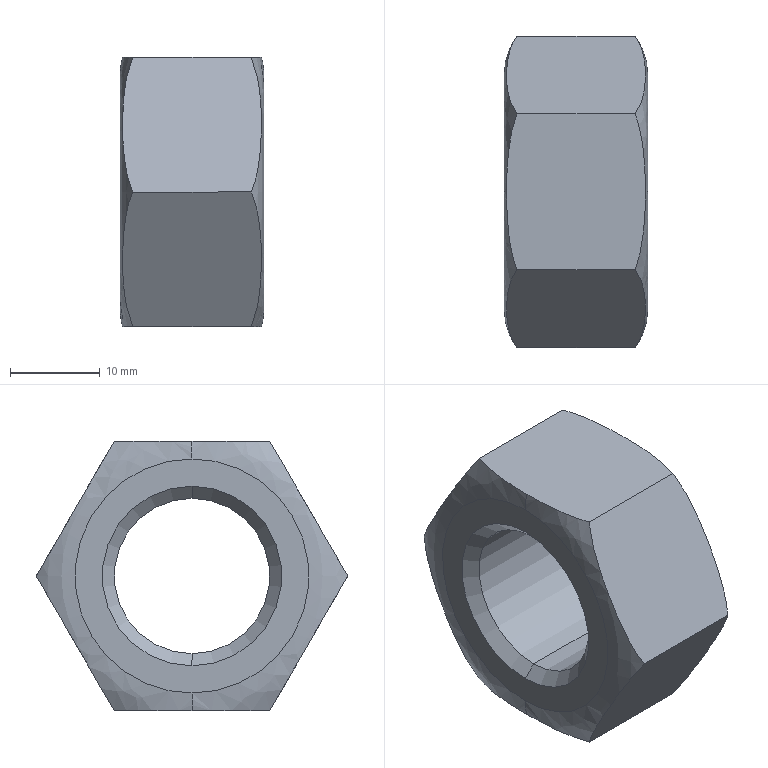Part | SolidWorks | features BaseBody 1 | 1 solid | 18 faces | box 16 x 34.641 x 30 mm | volume 8496 mm3 | plane 8 | spline 4 | cone 4 | cylinder 2 | commonest cylinder face diameters 17.294 x2
STEP:
#1=CARTESIAN_POINT('',(1.401,-8.66,15.));
#2=VERTEX_POINT('',#1);
#3=CARTESIAN_POINT('',(0.2735,0.,15.));
#4=VERTEX_POINT('',#3);
#5=CARTESIAN_POINT('',(1.401,-8.66,15.));
#6=CARTESIAN_POINT('',(1.148,-7.966,15.));
#7=CARTESIAN_POINT('',(0.9589,-7.26,15.));
#8=CARTESIAN_POINT('',(0.6645,-5.832,15.));
#9=CARTESIAN_POINT('',(0.5592,-5.11,15.));
#10=CARTESIAN_POINT('',(0.4034,-3.657,15.));
#11=CARTESIAN_POINT('',(0.3528,-2.924,15.));
#12=CARTESIAN_POINT('',(0.2879,-1.461,15.));
#13=CARTESIAN_POINT('',(0.2735,-0.73,15.));
#14=CARTESIAN_POINT('',(0.2735,0.,15.));
#15=B_SPLINE_CURVE_WITH_KNOTS('',3,(#5,#6,#7,#8,#9,#10,#11,#12,#13,#14),.UNSPECIFIED.,.F.,.F.,(4,2,2,2,4),(0.,0.002186,0.004373,0.006559,0.008745),.UNSPECIFIED.);
#16=EDGE_CURVE('',#2,#4,#15,.T.);
#17=ORIENTED_EDGE('',*,*,#16,.T.);
#18=CARTESIAN_POINT('',(0.,0.,13.021));
#19=VERTEX_POINT('',#18);
#20=CARTESIAN_POINT('',(7.3,0.,13.021));
#21=DIRECTION('',(0.,-1.,0.));
#22=DIRECTION('',(0.,0.,1.));
#23=AXIS2_PLACEMENT_3D('',#20,#21,#22);
#24=CIRCLE('',#23,7.3);
#25=EDGE_CURVE('',#4,#19,#24,.T.);
#26=ORIENTED_EDGE('',*,*,#25,.T.);
#27=CARTESIAN_POINT('',(0.,0.,-13.021));
#28=VERTEX_POINT('',#27);
#29=CARTESIAN_POINT('',(0.,0.,-13.021));
#30=CARTESIAN_POINT('',(0.,-0.3981,-13.021));
#31=CARTESIAN_POINT('',(0.,-0.9928,-12.993));
#32=CARTESIAN_POINT('',(0.,-1.682,-12.914));
#33=CARTESIAN_POINT('',(0.,-2.026,-12.863));
#34=CARTESIAN_POINT('',(0.,-2.198,-12.834));
#35=CARTESIAN_POINT('',(0.,-2.271,-12.821));
#36=CARTESIAN_POINT('',(0.,-2.32,-12.812));
#37=CARTESIAN_POINT('',(0.,-2.343,-12.808));
#38=CARTESIAN_POINT('',(0.,-2.784,-12.726));
#39=CARTESIAN_POINT('',(0.,-3.399,-12.582));
#40=CARTESIAN_POINT('',(0.,-4.101,-12.361));
#41=CARTESIAN_POINT('',(0.,-4.448,-12.238));
#42=CARTESIAN_POINT('',(0.,-4.596,-12.183));
#43=CARTESIAN_POINT('',(0.,-4.694,-12.145));
#44=CARTESIAN_POINT('',(0.,-4.742,-12.127));
#45=CARTESIAN_POINT('',(0.,-5.202,-11.944));
#46=CARTESIAN_POINT('',(0.,-5.8,-11.672));
#47=CARTESIAN_POINT('',(0.,-6.471,-11.302));
#48=CARTESIAN_POINT('',(0.,-6.8,-11.105));
#49=CARTESIAN_POINT('',(0.,-6.94,-11.017));
#50=CARTESIAN_POINT('',(0.,-7.033,-10.958));
#51=CARTESIAN_POINT('',(0.,-7.078,-10.929));
#52=CARTESIAN_POINT('',(0.,-7.877,-10.406));
#53=CARTESIAN_POINT('',(0.,-8.572,-9.842));
#54=CARTESIAN_POINT('',(0.,-9.525,-8.889));
#55=CARTESIAN_POINT('',(0.,-9.974,-8.391));
#56=CARTESIAN_POINT('',(0.,-10.452,-7.771));
#57=CARTESIAN_POINT('',(0.,-10.679,-7.451));
#58=CARTESIAN_POINT('',(0.,-10.774,-7.312));
#59=CARTESIAN_POINT('',(0.,-10.836,-7.219));
#60=CARTESIAN_POINT('',(0.,-10.868,-7.171));
#61=CARTESIAN_POINT('',(0.,-11.139,-6.757));
#62=CARTESIAN_POINT('',(0.,-11.47,-6.189));
#63=CARTESIAN_POINT('',(0.,-11.806,-5.5));
#64=CARTESIAN_POINT('',(0.,-11.96,-5.149));
#65=CARTESIAN_POINT('',(0.,-12.034,-4.971));
#66=CARTESIAN_POINT('',(0.,-12.065,-4.895));
#67=CARTESIAN_POINT('',(0.,-12.086,-4.844));
#68=CARTESIAN_POINT('',(0.,-12.097,-4.817));
#69=CARTESIAN_POINT('',(0.,-12.262,-4.4));
#70=CARTESIAN_POINT('',(0.,-12.465,-3.803));
#71=CARTESIAN_POINT('',(0.,-12.651,-3.091));
#72=CARTESIAN_POINT('',(0.,-12.732,-2.731));
#73=CARTESIAN_POINT('',(0.,-12.768,-2.551));
#74=CARTESIAN_POINT('',(0.,-12.784,-2.473));
#75=CARTESIAN_POINT('',(0.,-12.793,-2.421));
#76=CARTESIAN_POINT('',(0.,-12.799,-2.394));
#77=CARTESIAN_POINT('',(0.,-12.948,-1.587));
#78=CARTESIAN_POINT('',(0.,-13.02,-0.796));
#79=CARTESIAN_POINT('',(0.,-13.021,0.398));
#80=CARTESIAN_POINT('',(0.,-12.993,0.9927));
#81=CARTESIAN_POINT('',(0.,-12.914,1.682));
#82=CARTESIAN_POINT('',(0.,-12.863,2.026));
#83=CARTESIAN_POINT('',(0.,-12.834,2.198));
#84=CARTESIAN_POINT('',(0.,-12.821,2.271));
#85=CARTESIAN_POINT('',(0.,-12.812,2.32));
#86=CARTESIAN_POINT('',(0.,-12.808,2.343));
#87=CARTESIAN_POINT('',(0.,-12.726,2.784));
#88=CARTESIAN_POINT('',(0.,-12.582,3.399));
#89=CARTESIAN_POINT('',(0.,-12.361,4.101));
#90=CARTESIAN_POINT('',(0.,-12.238,4.448));
#91=CARTESIAN_POINT('',(0.,-12.183,4.596));
#92=CARTESIAN_POINT('',(0.,-12.145,4.694));
#93=CARTESIAN_POINT('',(0.,-12.127,4.742));
#94=CARTESIAN_POINT('',(0.,-11.944,5.202));
#95=CARTESIAN_POINT('',(0.,-11.672,5.8));
#96=CARTESIAN_POINT('',(0.,-11.302,6.471));
#97=CARTESIAN_POINT('',(0.,-11.105,6.8));
#98=CARTESIAN_POINT('',(0.,-11.017,6.94));
#99=CARTESIAN_POINT('',(0.,-10.958,7.033));
#100=CARTESIAN_POINT('',(0.,-10.929,7.078));
#101=CARTESIAN_POINT('',(0.,-10.406,7.877));
#102=CARTESIAN_POINT('',(0.,-9.842,8.572));
#103=CARTESIAN_POINT('',(0.,-8.889,9.525));
#104=CARTESIAN_POINT('',(0.,-8.391,9.974));
#105=CARTESIAN_POINT('',(0.,-7.771,10.452));
#106=CARTESIAN_POINT('',(0.,-7.451,10.679));
#107=CARTESIAN_POINT('',(0.,-7.312,10.774));
#108=CARTESIAN_POINT('',(0.,-7.219,10.836));
#109=CARTESIAN_POINT('',(0.,-7.171,10.868));
#110=CARTESIAN_POINT('',(0.,-6.757,11.139));
#111=CARTESIAN_POINT('',(0.,-6.189,11.47));
#112=CARTESIAN_POINT('',(0.,-5.5,11.806));
#113=CARTESIAN_POINT('',(0.,-5.149,11.96));
#114=CARTESIAN_POINT('',(0.,-4.971,12.034));
#115=CARTESIAN_POINT('',(0.,-4.895,12.065));
#116=CARTESIAN_POINT('',(0.,-4.844,12.086));
#117=CARTESIAN_POINT('',(0.,-4.817,12.097));
#118=CARTESIAN_POINT('',(0.,-4.4,12.262));
#119=CARTESIAN_POINT('',(0.,-3.803,12.465));
#120=CARTESIAN_POINT('',(0.,-3.091,12.651));
#121=CARTESIAN_POINT('',(0.,-2.731,12.732));
#122=CARTESIAN_POINT('',(0.,-2.551,12.768));
#123=CARTESIAN_POINT('',(0.,-2.473,12.784));
#124=CARTESIAN_POINT('',(0.,-2.421,12.793));
#125=CARTESIAN_POINT('',(0.,-2.394,12.799));
#126=CARTESIAN_POINT('',(0.,-1.587,12.948));
#127=CARTESIAN_POINT('',(0.,-0.796,13.02));
#128=CARTESIAN_POINT('',(0.,0.,13.021));
#129=B_SPLINE_CURVE_WITH_KNOTS('',3,(#29,#30,#31,#32,#33,#34,#35,#36,#37,#38,#39,#40,#41,#42,#43,#44,#45,#46,#47,#48,#49,#50,#51,#52,#53,#54,#55,#56,#57,#58,#59,#60,#61,#62,#63,#64,#65,#66,#67,#68,#69,#70,#71,#72,#73,#74,#75,#76,#77,#78,#79,#80,#81,#82,#83,#84,#85,#86,#87,#88,#89,#90,#91,#92,#93,#94,#95,#96,#97,#98,#99,#100,#101,#102,#103,#104,#105,#106,#107,#108,#109,#110,#111,#112,#113,#114,#115,#116,#117,#118,#119,#120,#121,#122,#123,#124,#125,#126,#127,#128),.UNSPECIFIED.,.F.,.F.,(4,1,1,1,1,2,2,1,1,1,2,2,1,1,1,2,2,2,1,1,1,2,2,1,1,1,1,2,2,1,1,1,1,2,2,2,1,1,1,1,2,2,1,1,1,2,2,1,1,1,2,2,2,1,1,1,2,2,1,1,1,1,2,2,1,1,1,1,2,2,4),(0.,0.01563,0.02344,0.02734,0.0293,0.03027,0.03125,0.04688,0.05469,0.05859,0.06055,0.0625,0.07813,0.08594,0.08984,0.0918,0.09375,0.125,0.1406,0.1484,0.1523,0.1543,0.1563,0.1719,0.1797,0.1836,0.1855,0.1865,0.1875,0.2031,0.2109,0.2148,0.2168,0.2178,0.2188,0.25,0.2656,0.2734,0.2773,0.2793,0.2803,0.2813,0.2969,0.3047,0.3086,0.3105,0.3125,0.3281,0.3359,0.3398,0.3418,0.3438,0.375,0.3906,0.3984,0.4023,0.4043,0.4063,0.4219,0.4297,0.4336,0.4355,0.4365,0.4375,0.4531,0.4609,0.4648,0.4668,0.4678,0.4688,0.5),.UNSPECIFIED.);
#130=EDGE_CURVE('',#28,#19,#129,.T.);
#131=ORIENTED_EDGE('',*,*,#130,.F.);
#132=CARTESIAN_POINT('',(0.2735,0.,-15.));
#133=VERTEX_POINT('',#132);
#134=CARTESIAN_POINT('',(7.3,0.,-13.021));
#135=DIRECTION('',(0.,1.,0.));
#136=DIRECTION('',(0.,0.,-1.));
#137=AXIS2_PLACEMENT_3D('',#134,#135,#136);
#138=CIRCLE('',#137,7.3);
#139=EDGE_CURVE('',#133,#28,#138,.T.);
#140=ORIENTED_EDGE('',*,*,#139,.F.);
#141=CARTESIAN_POINT('',(1.401,-8.66,-15.));
#142=VERTEX_POINT('',#141);
#143=CARTESIAN_POINT('',(0.2735,0.,-15.));
#144=CARTESIAN_POINT('',(0.2735,-0.7289,-15.));
#145=CARTESIAN_POINT('',(0.2879,-1.457,-15.));
#146=CARTESIAN_POINT('',(0.3521,-2.912,-15.));
#147=CARTESIAN_POINT('',(0.4019,-3.638,-15.));
#148=CARTESIAN_POINT('',(0.5565,-5.089,-15.));
#149=CARTESIAN_POINT('',(0.6611,-5.813,-15.));
#150=CARTESIAN_POINT('',(0.9579,-7.257,-15.));
#151=CARTESIAN_POINT('',(1.148,-7.967,-15.));
#152=CARTESIAN_POINT('',(1.401,-8.66,-15.));
#153=B_SPLINE_CURVE_WITH_KNOTS('',3,(#143,#144,#145,#146,#147,#148,#149,#150,#151,#152),.UNSPECIFIED.,.F.,.F.,(4,2,2,2,4),(0.008745,0.01093,0.01311,0.01529,0.01748),.UNSPECIFIED.);
#154=EDGE_CURVE('',#133,#142,#153,.T.);
#155=ORIENTED_EDGE('',*,*,#154,.T.);
#156=CARTESIAN_POINT('',(1.401,-17.321,0.));
#157=VERTEX_POINT('',#156);
#158=CARTESIAN_POINT('',(1.401,-8.66,-15.));
#159=CARTESIAN_POINT('',(1.148,-9.007,-14.399));
#160=CARTESIAN_POINT('',(0.9592,-9.36,-13.788));
#161=CARTESIAN_POINT('',(0.6649,-10.073,-12.552));
#162=CARTESIAN_POINT('',(0.5596,-10.434,-11.928));
#163=CARTESIAN_POINT('',(0.4037,-11.16,-10.67));
#164=CARTESIAN_POINT('',(0.3531,-11.526,-10.036));
#165=CARTESIAN_POINT('',(0.2881,-12.257,-8.77));
#166=CARTESIAN_POINT('',(0.2736,-12.622,-8.138));
#167=CARTESIAN_POINT('',(0.2734,-13.352,-6.874));
#168=CARTESIAN_POINT('',(0.2878,-13.716,-6.243));
#169=CARTESIAN_POINT('',(0.3518,-14.444,-4.982));
#170=CARTESIAN_POINT('',(0.4016,-14.808,-4.353));
#171=CARTESIAN_POINT('',(0.5561,-15.533,-3.095));
#172=CARTESIAN_POINT('',(0.6607,-15.896,-2.468));
#173=CARTESIAN_POINT('',(0.9576,-16.618,-1.216));
#174=CARTESIAN_POINT('',(1.148,-16.974,-0.6006));
#175=CARTESIAN_POINT('',(1.401,-17.321,0.));
#176=B_SPLINE_CURVE_WITH_KNOTS('',3,(#158,#159,#160,#161,#162,#163,#164,#165,#166,#167,#168,#169,#170,#171,#172,#173,#174,#175),.UNSPECIFIED.,.F.,.F.,(4,2,2,2,2,2,2,2,4),(0.,0.002185,0.004369,0.006554,0.008739,0.01092,0.01311,0.01529,0.01748),.UNSPECIFIED.);
#177=EDGE_CURVE('',#142,#157,#176,.T.);
#178=ORIENTED_EDGE('',*,*,#177,.T.);
#179=CARTESIAN_POINT('',(1.401,-17.321,0.));
#180=CARTESIAN_POINT('',(1.148,-16.974,0.6009));
#181=CARTESIAN_POINT('',(0.9592,-16.621,1.212));
#182=CARTESIAN_POINT('',(0.6649,-15.907,2.448));
#183=CARTESIAN_POINT('',(0.5596,-15.547,3.072));
#184=CARTESIAN_POINT('',(0.4037,-14.821,4.33));
#185=CARTESIAN_POINT('',(0.3531,-14.454,4.964));
#186=CARTESIAN_POINT('',(0.2881,-13.723,6.23));
#187=CARTESIAN_POINT('',(0.2736,-13.358,6.862));
#188=CARTESIAN_POINT('',(0.2734,-12.629,8.126));
#189=CARTESIAN_POINT('',(0.2878,-12.265,8.757));
#190=CARTESIAN_POINT('',(0.3518,-11.537,10.018));
#191=CARTESIAN_POINT('',(0.4016,-11.173,10.647));
#192=CARTESIAN_POINT('',(0.5561,-10.447,11.905));
#193=CARTESIAN_POINT('',(0.6607,-10.085,12.532));
#194=CARTESIAN_POINT('',(0.9576,-9.363,13.784));
#195=CARTESIAN_POINT('',(1.148,-9.007,14.399));
#196=CARTESIAN_POINT('',(1.401,-8.66,15.));
#197=B_SPLINE_CURVE_WITH_KNOTS('',3,(#179,#180,#181,#182,#183,#184,#185,#186,#187,#188,#189,#190,#191,#192,#193,#194,#195,#196),.UNSPECIFIED.,.F.,.F.,(4,2,2,2,2,2,2,2,4),(0.,0.002185,0.004369,0.006554,0.008739,0.01092,0.01311,0.01529,0.01748),.UNSPECIFIED.);
#198=EDGE_CURVE('',#157,#2,#197,.T.);
#199=ORIENTED_EDGE('',*,*,#198,.T.);
#200=EDGE_LOOP('',(#17,#26,#131,#140,#155,#178,#199));
#201=FACE_OUTER_BOUND('',#200,.T.);
#202=CARTESIAN_POINT('',(1.417,0.,17.343));
#203=CARTESIAN_POINT('',(1.417,-34.686,17.343));
#204=CARTESIAN_POINT('',(1.417,-34.686,-17.343));
#205=CARTESIAN_POINT('',(1.417,0.,-17.343));
#206=CARTESIAN_POINT('',(0.4886,0.,16.079));
#207=CARTESIAN_POINT('',(0.4886,-32.158,16.079));
#208=CARTESIAN_POINT('',(0.4886,-32.158,-16.079));
#209=CARTESIAN_POINT('',(0.4886,0.,-16.079));
#210=CARTESIAN_POINT('',(0.,0.,14.589));
#211=CARTESIAN_POINT('',(0.,-29.178,14.589));
#212=CARTESIAN_POINT('',(0.,-29.178,-14.589));
#213=CARTESIAN_POINT('',(0.,0.,-14.589));
#214=CARTESIAN_POINT('',(0.,0.,13.021));
#215=CARTESIAN_POINT('',(0.,-26.041,13.021));
#216=CARTESIAN_POINT('',(0.,-26.041,-13.021));
#217=CARTESIAN_POINT('',(0.,0.,-13.021));
#218=(BOUNDED_SURFACE()B_SPLINE_SURFACE(3,3,((#202,#203,#204,#205),(#206,#207,#208,#209),(#210,#211,#212,#213),(#214,#215,#216,#217)),.UNSPECIFIED.,.F.,.F.,.F.)B_SPLINE_SURFACE_WITH_KNOTS((4,4),(4,4),(0.,1.),(0.,1.),.UNSPECIFIED.)GEOMETRIC_REPRESENTATION_ITEM()RATIONAL_B_SPLINE_SURFACE(((1.,0.3333,0.3333,1.),(0.9668,0.3223,0.3223,0.9668),(0.9668,0.3223,0.3223,0.9668),(1.,0.3333,0.3333,1.)))REPRESENTATION_ITEM('')SURFACE());
#219=ADVANCED_FACE('',(#201),#218,.T.);
#220=CARTESIAN_POINT('',(16.,0.,13.021));
#221=VERTEX_POINT('',#220);
#222=CARTESIAN_POINT('',(16.,0.,-13.021));
#223=VERTEX_POINT('',#222);
#224=CARTESIAN_POINT('',(16.,0.,13.021));
#225=CARTESIAN_POINT('',(16.,-0.398,13.021));
#226=CARTESIAN_POINT('',(16.,-0.9927,12.993));
#227=CARTESIAN_POINT('',(16.,-1.682,12.914));
#228=CARTESIAN_POINT('',(16.,-2.026,12.863));
#229=CARTESIAN_POINT('',(16.,-2.198,12.834));
#230=CARTESIAN_POINT('',(16.,-2.271,12.821));
#231=CARTESIAN_POINT('',(16.,-2.32,12.812));
#232=CARTESIAN_POINT('',(16.,-2.343,12.808));
#233=CARTESIAN_POINT('',(16.,-2.784,12.726));
#234=CARTESIAN_POINT('',(16.,-3.399,12.582));
#235=CARTESIAN_POINT('',(16.,-4.101,12.361));
#236=CARTESIAN_POINT('',(16.,-4.448,12.238));
#237=CARTESIAN_POINT('',(16.,-4.596,12.183));
#238=CARTESIAN_POINT('',(16.,-4.694,12.145));
#239=CARTESIAN_POINT('',(16.,-4.742,12.127));
#240=CARTESIAN_POINT('',(16.,-5.202,11.944));
#241=CARTESIAN_POINT('',(16.,-5.8,11.672));
#242=CARTESIAN_POINT('',(16.,-6.471,11.302));
#243=CARTESIAN_POINT('',(16.,-6.8,11.105));
#244=CARTESIAN_POINT('',(16.,-6.94,11.017));
#245=CARTESIAN_POINT('',(16.,-7.033,10.958));
#246=CARTESIAN_POINT('',(16.,-7.078,10.929));
#247=CARTESIAN_POINT('',(16.,-7.877,10.406));
#248=CARTESIAN_POINT('',(16.,-8.572,9.842));
#249=CARTESIAN_POINT('',(16.,-9.525,8.889));
#250=CARTESIAN_POINT('',(16.,-9.974,8.391));
#251=CARTESIAN_POINT('',(16.,-10.452,7.771));
#252=CARTESIAN_POINT('',(16.,-10.679,7.451));
#253=CARTESIAN_POINT('',(16.,-10.774,7.312));
#254=CARTESIAN_POINT('',(16.,-10.836,7.219));
#255=CARTESIAN_POINT('',(16.,-10.868,7.171));
#256=CARTESIAN_POINT('',(16.,-11.139,6.757));
#257=CARTESIAN_POINT('',(16.,-11.47,6.189));
#258=CARTESIAN_POINT('',(16.,-11.806,5.5));
#259=CARTESIAN_POINT('',(16.,-11.96,5.149));
#260=CARTESIAN_POINT('',(16.,-12.034,4.971));
#261=CARTESIAN_POINT('',(16.,-12.065,4.895));
#262=CARTESIAN_POINT('',(16.,-12.086,4.844));
#263=CARTESIAN_POINT('',(16.,-12.097,4.817));
#264=CARTESIAN_POINT('',(16.,-12.262,4.4));
#265=CARTESIAN_POINT('',(16.,-12.465,3.803));
#266=CARTESIAN_POINT('',(16.,-12.651,3.091));
#267=CARTESIAN_POINT('',(16.,-12.732,2.731));
#268=CARTESIAN_POINT('',(16.,-12.768,2.551));
#269=CARTESIAN_POINT('',(16.,-12.784,2.473));
#270=CARTESIAN_POINT('',(16.,-12.793,2.421));
#271=CARTESIAN_POINT('',(16.,-12.799,2.394));
#272=CARTESIAN_POINT('',(16.,-12.948,1.587));
#273=CARTESIAN_POINT('',(16.,-13.02,0.796));
#274=CARTESIAN_POINT('',(16.,-13.021,-0.398));
#275=CARTESIAN_POINT('',(16.,-12.993,-0.9927));
#276=CARTESIAN_POINT('',(16.,-12.914,-1.682));
#277=CARTESIAN_POINT('',(16.,-12.863,-2.026));
#278=CARTESIAN_POINT('',(16.,-12.834,-2.198));
#279=CARTESIAN_POINT('',(16.,-12.821,-2.271));
#280=CARTESIAN_POINT('',(16.,-12.812,-2.32));
#281=CARTESIAN_POINT('',(16.,-12.808,-2.343));
#282=CARTESIAN_POINT('',(16.,-12.726,-2.784));
#283=CARTESIAN_POINT('',(16.,-12.582,-3.399));
#284=CARTESIAN_POINT('',(16.,-12.361,-4.101));
#285=CARTESIAN_POINT('',(16.,-12.238,-4.448));
#286=CARTESIAN_POINT('',(16.,-12.183,-4.596));
#287=CARTESIAN_POINT('',(16.,-12.145,-4.694));
#288=CARTESIAN_POINT('',(16.,-12.127,-4.742));
#289=CARTESIAN_POINT('',(16.,-11.944,-5.202));
#290=CARTESIAN_POINT('',(16.,-11.672,-5.8));
#291=CARTESIAN_POINT('',(16.,-11.302,-6.471));
#292=CARTESIAN_POINT('',(16.,-11.105,-6.8));
#293=CARTESIAN_POINT('',(16.,-11.017,-6.94));
#294=CARTESIAN_POINT('',(16.,-10.958,-7.033));
#295=CARTESIAN_POINT('',(16.,-10.929,-7.078));
#296=CARTESIAN_POINT('',(16.,-10.406,-7.877));
#297=CARTESIAN_POINT('',(16.,-9.842,-8.572));
#298=CARTESIAN_POINT('',(16.,-8.889,-9.525));
#299=CARTESIAN_POINT('',(16.,-8.391,-9.974));
#300=CARTESIAN_POINT('',(16.,-7.771,-10.452));
#301=CARTESIAN_POINT('',(16.,-7.451,-10.679));
#302=CARTESIAN_POINT('',(16.,-7.312,-10.774));
#303=CARTESIAN_POINT('',(16.,-7.219,-10.836));
#304=CARTESIAN_POINT('',(16.,-7.171,-10.868));
#305=CARTESIAN_POINT('',(16.,-6.757,-11.139));
#306=CARTESIAN_POINT('',(16.,-6.189,-11.47));
#307=CARTESIAN_POINT('',(16.,-5.5,-11.806));
#308=CARTESIAN_POINT('',(16.,-5.149,-11.96));
#309=CARTESIAN_POINT('',(16.,-4.971,-12.034));
#310=CARTESIAN_POINT('',(16.,-4.895,-12.065));
#311=CARTESIAN_POINT('',(16.,-4.844,-12.086));
#312=CARTESIAN_POINT('',(16.,-4.817,-12.097));
#313=CARTESIAN_POINT('',(16.,-4.4,-12.262));
#314=CARTESIAN_POINT('',(16.,-3.803,-12.465));
#315=CARTESIAN_POINT('',(16.,-3.091,-12.651));
#316=CARTESIAN_POINT('',(16.,-2.731,-12.732));
#317=CARTESIAN_POINT('',(16.,-2.551,-12.768));
#318=CARTESIAN_POINT('',(16.,-2.473,-12.784));
#319=CARTESIAN_POINT('',(16.,-2.421,-12.793));
#320=CARTESIAN_POINT('',(16.,-2.394,-12.799));
#321=CARTESIAN_POINT('',(16.,-1.586,-12.948));
#322=CARTESIAN_POINT('',(16.,-0.7966,-13.021));
#323=CARTESIAN_POINT('',(16.,0.,-13.021));
#324=B_SPLINE_CURVE_WITH_KNOTS('',3,(#224,#225,#226,#227,#228,#229,#230,#231,#232,#233,#234,#235,#236,#237,#238,#239,#240,#241,#242,#243,#244,#245,#246,#247,#248,#249,#250,#251,#252,#253,#254,#255,#256,#257,#258,#259,#260,#261,#262,#263,#264,#265,#266,#267,#268,#269,#270,#271,#272,#273,#274,#275,#276,#277,#278,#279,#280,#281,#282,#283,#284,#285,#286,#287,#288,#289,#290,#291,#292,#293,#294,#295,#296,#297,#298,#299,#300,#301,#302,#303,#304,#305,#306,#307,#308,#309,#310,#311,#312,#313,#314,#315,#316,#317,#318,#319,#320,#321,#322,#323),.UNSPECIFIED.,.F.,.F.,(4,1,1,1,1,2,2,1,1,1,2,2,1,1,1,2,2,2,1,1,1,2,2,1,1,1,1,2,2,1,1,1,1,2,2,2,1,1,1,1,2,2,1,1,1,2,2,1,1,1,2,2,2,1,1,1,2,2,1,1,1,1,2,2,1,1,1,1,2,2,4),(0.5,0.5156,0.5234,0.5273,0.5293,0.5303,0.5312,0.5469,0.5547,0.5586,0.5605,0.5625,0.5781,0.5859,0.5898,0.5918,0.5937,0.625,0.6406,0.6484,0.6523,0.6543,0.6562,0.6719,0.6797,0.6836,0.6855,0.6865,0.6875,0.7031,0.7109,0.7148,0.7168,0.7178,0.7187,0.75,0.7656,0.7734,0.7773,0.7793,0.7803,0.7812,0.7969,0.8047,0.8086,0.8105,0.8125,0.8281,0.8359,0.8398,0.8418,0.8437,0.875,0.8906,0.8984,0.9023,0.9043,0.9062,0.9219,0.9297,0.9336,0.9355,0.9365,0.9375,0.9531,0.9609,0.9648,0.9668,0.9678,0.9687,1.),.UNSPECIFIED.);
#325=EDGE_CURVE('',#221,#223,#324,.T.);
#326=ORIENTED_EDGE('',*,*,#325,.F.);
#327=CARTESIAN_POINT('',(15.726,0.,15.));
#328=VERTEX_POINT('',#327);
#329=CARTESIAN_POINT('',(8.7,0.,13.021));
#330=DIRECTION('',(0.,-1.,0.));
#331=DIRECTION('',(0.,0.,1.));
#332=AXIS2_PLACEMENT_3D('',#329,#330,#331);
#333=CIRCLE('',#332,7.3);
#334=EDGE_CURVE('',#221,#328,#333,.T.);
#335=ORIENTED_EDGE('',*,*,#334,.T.);
#336=CARTESIAN_POINT('',(14.599,-8.66,15.));
#337=VERTEX_POINT('',#336);
#338=CARTESIAN_POINT('',(15.726,0.,15.));
#339=CARTESIAN_POINT('',(15.726,-0.7289,15.));
#340=CARTESIAN_POINT('',(15.712,-1.457,15.));
#341=CARTESIAN_POINT('',(15.648,-2.912,15.));
#342=CARTESIAN_POINT('',(15.598,-3.638,15.));
#343=CARTESIAN_POINT('',(15.444,-5.089,15.));
#344=CARTESIAN_POINT('',(15.339,-5.813,15.));
#345=CARTESIAN_POINT('',(15.042,-7.257,15.));
#346=CARTESIAN_POINT('',(14.852,-7.967,15.));
#347=CARTESIAN_POINT('',(14.599,-8.66,15.));
#348=B_SPLINE_CURVE_WITH_KNOTS('',3,(#338,#339,#340,#341,#342,#343,#344,#345,#346,#347),.UNSPECIFIED.,.F.,.F.,(4,2,2,2,4),(0.008745,0.01093,0.01311,0.01529,0.01748),.UNSPECIFIED.);
#349=EDGE_CURVE('',#328,#337,#348,.T.);
#350=ORIENTED_EDGE('',*,*,#349,.T.);
#351=CARTESIAN_POINT('',(14.599,-17.321,0.));
#352=VERTEX_POINT('',#351);
#353=CARTESIAN_POINT('',(14.599,-8.66,15.));
#354=CARTESIAN_POINT('',(14.852,-9.007,14.399));
#355=CARTESIAN_POINT('',(15.041,-9.36,13.788));
#356=CARTESIAN_POINT('',(15.335,-10.073,12.552));
#357=CARTESIAN_POINT('',(15.44,-10.434,11.928));
#358=CARTESIAN_POINT('',(15.596,-11.16,10.67));
#359=CARTESIAN_POINT('',(15.647,-11.526,10.036));
#360=CARTESIAN_POINT('',(15.712,-12.257,8.77));
#361=CARTESIAN_POINT('',(15.726,-12.622,8.138));
#362=CARTESIAN_POINT('',(15.727,-13.352,6.874));
#363=CARTESIAN_POINT('',(15.712,-13.716,6.243));
#364=CARTESIAN_POINT('',(15.648,-14.444,4.982));
#365=CARTESIAN_POINT('',(15.598,-14.808,4.353));
#366=CARTESIAN_POINT('',(15.444,-15.533,3.095));
#367=CARTESIAN_POINT('',(15.339,-15.896,2.468));
#368=CARTESIAN_POINT('',(15.042,-16.618,1.216));
#369=CARTESIAN_POINT('',(14.852,-16.974,0.6006));
#370=CARTESIAN_POINT('',(14.599,-17.321,0.));
#371=B_SPLINE_CURVE_WITH_KNOTS('',3,(#353,#354,#355,#356,#357,#358,#359,#360,#361,#362,#363,#364,#365,#366,#367,#368,#369,#370),.UNSPECIFIED.,.F.,.F.,(4,2,2,2,2,2,2,2,4),(0.,0.002185,0.004369,0.006554,0.008739,0.01092,0.01311,0.01529,0.01748),.UNSPECIFIED.);
#372=EDGE_CURVE('',#337,#352,#371,.T.);
#373=ORIENTED_EDGE('',*,*,#372,.T.);
#374=CARTESIAN_POINT('',(14.599,-8.66,-15.));
#375=VERTEX_POINT('',#374);
#376=CARTESIAN_POINT('',(14.599,-17.321,0.));
#377=CARTESIAN_POINT('',(14.852,-16.974,-0.6009));
#378=CARTESIAN_POINT('',(15.041,-16.621,-1.212));
#379=CARTESIAN_POINT('',(15.335,-15.907,-2.448));
#380=CARTESIAN_POINT('',(15.44,-15.547,-3.072));
#381=CARTESIAN_POINT('',(15.596,-14.821,-4.33));
#382=CARTESIAN_POINT('',(15.647,-14.454,-4.964));
#383=CARTESIAN_POINT('',(15.712,-13.723,-6.23));
#384=CARTESIAN_POINT('',(15.726,-13.358,-6.862));
#385=CARTESIAN_POINT('',(15.727,-12.629,-8.126));
#386=CARTESIAN_POINT('',(15.712,-12.265,-8.757));
#387=CARTESIAN_POINT('',(15.648,-11.537,-10.018));
#388=CARTESIAN_POINT('',(15.598,-11.173,-10.647));
#389=CARTESIAN_POINT('',(15.444,-10.447,-11.905));
#390=CARTESIAN_POINT('',(15.339,-10.085,-12.532));
#391=CARTESIAN_POINT('',(15.042,-9.363,-13.784));
#392=CARTESIAN_POINT('',(14.852,-9.007,-14.399));
#393=CARTESIAN_POINT('',(14.599,-8.66,-15.));
#394=B_SPLINE_CURVE_WITH_KNOTS('',3,(#376,#377,#378,#379,#380,#381,#382,#383,#384,#385,#386,#387,#388,#389,#390,#391,#392,#393),.UNSPECIFIED.,.F.,.F.,(4,2,2,2,2,2,2,2,4),(0.,0.002185,0.004369,0.006554,0.008739,0.01092,0.01311,0.01529,0.01748),.UNSPECIFIED.);
#395=EDGE_CURVE('',#352,#375,#394,.T.);
#396=ORIENTED_EDGE('',*,*,#395,.T.);
#397=CARTESIAN_POINT('',(15.726,0.,-15.));
#398=VERTEX_POINT('',#397);
#399=CARTESIAN_POINT('',(14.599,-8.66,-15.));
#400=CARTESIAN_POINT('',(14.852,-7.966,-15.));
#401=CARTESIAN_POINT('',(15.041,-7.26,-15.));
#402=CARTESIAN_POINT('',(15.336,-5.832,-15.));
#403=CARTESIAN_POINT('',(15.441,-5.11,-15.));
#404=CARTESIAN_POINT('',(15.597,-3.657,-15.));
#405=CARTESIAN_POINT('',(15.647,-2.924,-15.));
#406=CARTESIAN_POINT('',(15.712,-1.461,-15.));
#407=CARTESIAN_POINT('',(15.726,-0.73,-15.));
#408=CARTESIAN_POINT('',(15.726,0.,-15.));
#409=B_SPLINE_CURVE_WITH_KNOTS('',3,(#399,#400,#401,#402,#403,#404,#405,#406,#407,#408),.UNSPECIFIED.,.F.,.F.,(4,2,2,2,4),(0.,0.002186,0.004373,0.006559,0.008745),.UNSPECIFIED.);
#410=EDGE_CURVE('',#375,#398,#409,.T.);
#411=ORIENTED_EDGE('',*,*,#410,.T.);
#412=CARTESIAN_POINT('',(8.7,0.,-13.021));
#413=DIRECTION('',(0.,1.,0.));
#414=DIRECTION('',(0.,0.,-1.));
#415=AXIS2_PLACEMENT_3D('',#412,#413,#414);
#416=CIRCLE('',#415,7.3);
#417=EDGE_CURVE('',#223,#398,#416,.T.);
#418=ORIENTED_EDGE('',*,*,#417,.F.);
#419=EDGE_LOOP('',(#326,#335,#350,#373,#396,#411,#418));
#420=FACE_OUTER_BOUND('',#419,.T.);
#421=CARTESIAN_POINT('',(16.,0.,13.021));
#422=CARTESIAN_POINT('',(16.,-26.041,13.021));
#423=CARTESIAN_POINT('',(16.,-26.041,-13.021));
#424=CARTESIAN_POINT('',(16.,0.,-13.021));
#425=CARTESIAN_POINT('',(16.,0.,14.589));
#426=CARTESIAN_POINT('',(16.,-29.178,14.589));
#427=CARTESIAN_POINT('',(16.,-29.178,-14.589));
#428=CARTESIAN_POINT('',(16.,0.,-14.589));
#429=CARTESIAN_POINT('',(15.511,0.,16.079));
#430=CARTESIAN_POINT('',(15.511,-32.158,16.079));
#431=CARTESIAN_POINT('',(15.511,-32.158,-16.079));
#432=CARTESIAN_POINT('',(15.511,0.,-16.079));
#433=CARTESIAN_POINT('',(14.583,0.,17.343));
#434=CARTESIAN_POINT('',(14.583,-34.686,17.343));
#435=CARTESIAN_POINT('',(14.583,-34.686,-17.343));
#436=CARTESIAN_POINT('',(14.583,0.,-17.343));
#437=(BOUNDED_SURFACE()B_SPLINE_SURFACE(3,3,((#421,#422,#423,#424),(#425,#426,#427,#428),(#429,#430,#431,#432),(#433,#434,#435,#436)),.UNSPECIFIED.,.F.,.F.,.F.)B_SPLINE_SURFACE_WITH_KNOTS((4,4),(4,4),(0.,1.),(0.,1.),.UNSPECIFIED.)GEOMETRIC_REPRESENTATION_ITEM()RATIONAL_B_SPLINE_SURFACE(((1.,0.3333,0.3333,1.),(0.9668,0.3223,0.3223,0.9668),(0.9668,0.3223,0.3223,0.9668),(1.,0.3333,0.3333,1.)))REPRESENTATION_ITEM('')SURFACE());
#438=ADVANCED_FACE('',(#420),#437,.T.);
#439=CARTESIAN_POINT('',(1.353,0.,8.647));
#440=VERTEX_POINT('',#439);
#441=CARTESIAN_POINT('',(1.353,0.,-8.647));
#442=VERTEX_POINT('',#441);
#443=CARTESIAN_POINT('',(1.353,0.,0.));
#444=DIRECTION('',(1.,0.,0.));
#445=DIRECTION('',(0.,0.,-1.));
#446=AXIS2_PLACEMENT_3D('',#443,#444,#445);
#447=CIRCLE('',#446,8.647);
#448=EDGE_CURVE('',#440,#442,#447,.T.);
#449=ORIENTED_EDGE('',*,*,#448,.F.);
#450=CARTESIAN_POINT('',(14.647,0.,8.647));
#451=VERTEX_POINT('',#450);
#452=CARTESIAN_POINT('',(34225.,0.,8.647));
#453=DIRECTION('',(1.,0.,0.));
#454=VECTOR('',#453,1000.);
#455=LINE('',#452,#454);
#456=EDGE_CURVE('',#440,#451,#455,.T.);
#457=ORIENTED_EDGE('',*,*,#456,.T.);
#458=CARTESIAN_POINT('',(14.647,0.,-8.647));
#459=VERTEX_POINT('',#458);
#460=CARTESIAN_POINT('',(14.647,0.,0.));
#461=DIRECTION('',(-1.,0.,0.));
#462=DIRECTION('',(0.,0.,-1.));
#463=AXIS2_PLACEMENT_3D('',#460,#461,#462);
#464=CIRCLE('',#463,8.647);
#465=EDGE_CURVE('',#459,#451,#464,.T.);
#466=ORIENTED_EDGE('',*,*,#465,.F.);
#467=CARTESIAN_POINT('',(34225.,0.,-8.647));
#468=DIRECTION('',(1.,0.,0.));
#469=VECTOR('',#468,1000.);
#470=LINE('',#467,#469);
#471=EDGE_CURVE('',#442,#459,#470,.T.);
#472=ORIENTED_EDGE('',*,*,#471,.F.);
#473=EDGE_LOOP('',(#449,#457,#466,#472));
#474=FACE_OUTER_BOUND('',#473,.T.);
#475=CARTESIAN_POINT('',(34225.,0.,0.));
#476=DIRECTION('',(1.,0.,0.));
#477=DIRECTION('',(0.,0.,-1.));
#478=AXIS2_PLACEMENT_3D('',#475,#476,#477);
#479=CYLINDRICAL_SURFACE('',#478,8.647);
#480=ADVANCED_FACE('',(#474),#479,.F.);
#481=ORIENTED_EDGE('',*,*,#448,.T.);
#482=CARTESIAN_POINT('',(0.,0.,-10.));
#483=VERTEX_POINT('',#482);
#484=CARTESIAN_POINT('',(0.,0.,-10.));
#485=DIRECTION('',(-0.7071,0.,-0.7071));
#486=VECTOR('',#485,1000.);
#487=LINE('',#484,#486);
#488=EDGE_CURVE('',#442,#483,#487,.T.);
#489=ORIENTED_EDGE('',*,*,#488,.T.);
#490=CARTESIAN_POINT('',(0.,0.,10.));
#491=VERTEX_POINT('',#490);
#492=CARTESIAN_POINT('',(0.,0.,0.));
#493=DIRECTION('',(1.,0.,0.));
#494=DIRECTION('',(0.,0.,1.));
#495=AXIS2_PLACEMENT_3D('',#492,#493,#494);
#496=CIRCLE('',#495,10.);
#497=EDGE_CURVE('',#491,#483,#496,.T.);
#498=ORIENTED_EDGE('',*,*,#497,.F.);
#499=CARTESIAN_POINT('',(0.,0.,10.));
#500=DIRECTION('',(-0.7071,0.,0.7071));
#501=VECTOR('',#500,1000.);
#502=LINE('',#499,#501);
#503=EDGE_CURVE('',#440,#491,#502,.T.);
#504=ORIENTED_EDGE('',*,*,#503,.F.);
#505=EDGE_LOOP('',(#481,#489,#498,#504));
#506=FACE_OUTER_BOUND('',#505,.T.);
#507=CARTESIAN_POINT('',(0.,0.,0.));
#508=DIRECTION('',(-1.,0.,0.));
#509=DIRECTION('',(0.,0.,1.));
#510=AXIS2_PLACEMENT_3D('',#507,#508,#509);
#511=CONICAL_SURFACE('',#510,10.,0.7854);
#512=ADVANCED_FACE('',(#506),#511,.F.);
#513=ORIENTED_EDGE('',*,*,#465,.T.);
#514=CARTESIAN_POINT('',(16.,0.,10.));
#515=VERTEX_POINT('',#514);
#516=CARTESIAN_POINT('',(16.,0.,10.));
#517=DIRECTION('',(0.7071,0.,0.7071));
#518=VECTOR('',#517,1000.);
#519=LINE('',#516,#518);
#520=EDGE_CURVE('',#451,#515,#519,.T.);
#521=ORIENTED_EDGE('',*,*,#520,.T.);
#522=CARTESIAN_POINT('',(16.,0.,-10.));
#523=VERTEX_POINT('',#522);
#524=CARTESIAN_POINT('',(16.,0.,0.));
#525=DIRECTION('',(-1.,0.,0.));
#526=DIRECTION('',(0.,0.,-1.));
#527=AXIS2_PLACEMENT_3D('',#524,#525,#526);
#528=CIRCLE('',#527,10.);
#529=EDGE_CURVE('',#523,#515,#528,.T.);
#530=ORIENTED_EDGE('',*,*,#529,.F.);
#531=CARTESIAN_POINT('',(16.,0.,-10.));
#532=DIRECTION('',(0.7071,0.,-0.7071));
#533=VECTOR('',#532,1000.);
#534=LINE('',#531,#533);
#535=EDGE_CURVE('',#459,#523,#534,.T.);
#536=ORIENTED_EDGE('',*,*,#535,.F.);
#537=EDGE_LOOP('',(#513,#521,#530,#536));
#538=FACE_OUTER_BOUND('',#537,.T.);
#539=CARTESIAN_POINT('',(16.,0.,0.));
#540=DIRECTION('',(1.,0.,0.));
#541=DIRECTION('',(0.,0.,-1.));
#542=AXIS2_PLACEMENT_3D('',#539,#540,#541);
#543=CONICAL_SURFACE('',#542,10.,0.7854);
#544=ADVANCED_FACE('',(#538),#543,.F.);
#545=ORIENTED_EDGE('',*,*,#456,.F.);
#546=CARTESIAN_POINT('',(1.353,0.,0.));
#547=DIRECTION('',(1.,0.,0.));
#548=DIRECTION('',(0.,0.,-1.));
#549=AXIS2_PLACEMENT_3D('',#546,#547,#548);
#550=CIRCLE('',#549,8.647);
#551=EDGE_CURVE('',#442,#440,#550,.T.);
#552=ORIENTED_EDGE('',*,*,#551,.F.);
#553=ORIENTED_EDGE('',*,*,#471,.T.);
#554=CARTESIAN_POINT('',(14.647,0.,0.));
#555=DIRECTION('',(-1.,0.,0.));
#556=DIRECTION('',(0.,0.,-1.));
#557=AXIS2_PLACEMENT_3D('',#554,#555,#556);
#558=CIRCLE('',#557,8.647);
#559=EDGE_CURVE('',#451,#459,#558,.T.);
#560=ORIENTED_EDGE('',*,*,#559,.F.);
#561=EDGE_LOOP('',(#545,#552,#553,#560));
#562=FACE_OUTER_BOUND('',#561,.T.);
#563=CARTESIAN_POINT('',(34225.,0.,0.));
#564=DIRECTION('',(1.,0.,0.));
#565=DIRECTION('',(0.,0.,-1.));
#566=AXIS2_PLACEMENT_3D('',#563,#564,#565);
#567=CYLINDRICAL_SURFACE('',#566,8.647);
#568=ADVANCED_FACE('',(#562),#567,.F.);
#569=ORIENTED_EDGE('',*,*,#488,.F.);
#570=ORIENTED_EDGE('',*,*,#551,.T.);
#571=ORIENTED_EDGE('',*,*,#503,.T.);
#572=CARTESIAN_POINT('',(0.,0.,0.));
#573=DIRECTION('',(1.,0.,0.));
#574=DIRECTION('',(0.,0.,1.));
#575=AXIS2_PLACEMENT_3D('',#572,#573,#574);
#576=CIRCLE('',#575,10.);
#577=EDGE_CURVE('',#483,#491,#576,.T.);
#578=ORIENTED_EDGE('',*,*,#577,.F.);
#579=EDGE_LOOP('',(#569,#570,#571,#578));
#580=FACE_OUTER_BOUND('',#579,.T.);
#581=CARTESIAN_POINT('',(0.,0.,0.));
#582=DIRECTION('',(-1.,0.,0.));
#583=DIRECTION('',(0.,0.,1.));
#584=AXIS2_PLACEMENT_3D('',#581,#582,#583);
#585=CONICAL_SURFACE('',#584,10.,0.7854);
#586=ADVANCED_FACE('',(#580),#585,.F.);
#587=ORIENTED_EDGE('',*,*,#520,.F.);
#588=ORIENTED_EDGE('',*,*,#559,.T.);
#589=ORIENTED_EDGE('',*,*,#535,.T.);
#590=CARTESIAN_POINT('',(16.,0.,0.));
#591=DIRECTION('',(-1.,0.,0.));
#592=DIRECTION('',(0.,0.,-1.));
#593=AXIS2_PLACEMENT_3D('',#590,#591,#592);
#594=CIRCLE('',#593,10.);
#595=EDGE_CURVE('',#515,#523,#594,.T.);
#596=ORIENTED_EDGE('',*,*,#595,.F.);
#597=EDGE_LOOP('',(#587,#588,#589,#596));
#598=FACE_OUTER_BOUND('',#597,.T.);
#599=CARTESIAN_POINT('',(16.,0.,0.));
#600=DIRECTION('',(1.,0.,0.));
#601=DIRECTION('',(0.,0.,-1.));
#602=AXIS2_PLACEMENT_3D('',#599,#600,#601);
#603=CONICAL_SURFACE('',#602,10.,0.7854);
#604=ADVANCED_FACE('',(#598),#603,.F.);
#605=ORIENTED_EDGE('',*,*,#130,.T.);
#606=CARTESIAN_POINT('',(0.,0.,13.021));
#607=CARTESIAN_POINT('',(0.,0.398,13.021));
#608=CARTESIAN_POINT('',(0.,0.9927,12.993));
#609=CARTESIAN_POINT('',(0.,1.682,12.914));
#610=CARTESIAN_POINT('',(0.,2.026,12.863));
#611=CARTESIAN_POINT('',(0.,2.198,12.834));
#612=CARTESIAN_POINT('',(0.,2.271,12.821));
#613=CARTESIAN_POINT('',(0.,2.32,12.812));
#614=CARTESIAN_POINT('',(0.,2.343,12.808));
#615=CARTESIAN_POINT('',(0.,2.784,12.726));
#616=CARTESIAN_POINT('',(0.,3.399,12.582));
#617=CARTESIAN_POINT('',(0.,4.101,12.361));
#618=CARTESIAN_POINT('',(0.,4.448,12.238));
#619=CARTESIAN_POINT('',(0.,4.596,12.183));
#620=CARTESIAN_POINT('',(0.,4.694,12.145));
#621=CARTESIAN_POINT('',(0.,4.742,12.127));
#622=CARTESIAN_POINT('',(0.,5.202,11.944));
#623=CARTESIAN_POINT('',(0.,5.8,11.672));
#624=CARTESIAN_POINT('',(0.,6.471,11.302));
#625=CARTESIAN_POINT('',(0.,6.8,11.105));
#626=CARTESIAN_POINT('',(0.,6.94,11.017));
#627=CARTESIAN_POINT('',(0.,7.033,10.958));
#628=CARTESIAN_POINT('',(0.,7.078,10.929));
#629=CARTESIAN_POINT('',(0.,7.877,10.406));
#630=CARTESIAN_POINT('',(0.,8.572,9.842));
#631=CARTESIAN_POINT('',(0.,9.525,8.889));
#632=CARTESIAN_POINT('',(0.,9.974,8.391));
#633=CARTESIAN_POINT('',(0.,10.452,7.771));
#634=CARTESIAN_POINT('',(0.,10.679,7.451));
#635=CARTESIAN_POINT('',(0.,10.774,7.312));
#636=CARTESIAN_POINT('',(0.,10.836,7.219));
#637=CARTESIAN_POINT('',(0.,10.868,7.171));
#638=CARTESIAN_POINT('',(0.,11.139,6.757));
#639=CARTESIAN_POINT('',(0.,11.47,6.189));
#640=CARTESIAN_POINT('',(0.,11.806,5.5));
#641=CARTESIAN_POINT('',(0.,11.96,5.149));
#642=CARTESIAN_POINT('',(0.,12.034,4.971));
#643=CARTESIAN_POINT('',(0.,12.065,4.895));
#644=CARTESIAN_POINT('',(0.,12.086,4.844));
#645=CARTESIAN_POINT('',(0.,12.097,4.817));
#646=CARTESIAN_POINT('',(0.,12.262,4.4));
#647=CARTESIAN_POINT('',(0.,12.465,3.803));
#648=CARTESIAN_POINT('',(0.,12.651,3.091));
#649=CARTESIAN_POINT('',(0.,12.732,2.731));
#650=CARTESIAN_POINT('',(0.,12.768,2.551));
#651=CARTESIAN_POINT('',(0.,12.784,2.473));
#652=CARTESIAN_POINT('',(0.,12.793,2.421));
#653=CARTESIAN_POINT('',(0.,12.799,2.394));
#654=CARTESIAN_POINT('',(0.,12.948,1.587));
#655=CARTESIAN_POINT('',(0.,13.02,0.796));
#656=CARTESIAN_POINT('',(0.,13.021,-0.398));
#657=CARTESIAN_POINT('',(0.,12.993,-0.9927));
#658=CARTESIAN_POINT('',(0.,12.914,-1.682));
#659=CARTESIAN_POINT('',(0.,12.863,-2.026));
#660=CARTESIAN_POINT('',(0.,12.834,-2.198));
#661=CARTESIAN_POINT('',(0.,12.821,-2.271));
#662=CARTESIAN_POINT('',(0.,12.812,-2.32));
#663=CARTESIAN_POINT('',(0.,12.808,-2.343));
#664=CARTESIAN_POINT('',(0.,12.726,-2.784));
#665=CARTESIAN_POINT('',(0.,12.582,-3.399));
#666=CARTESIAN_POINT('',(0.,12.361,-4.101));
#667=CARTESIAN_POINT('',(0.,12.238,-4.448));
#668=CARTESIAN_POINT('',(0.,12.183,-4.596));
#669=CARTESIAN_POINT('',(0.,12.145,-4.694));
#670=CARTESIAN_POINT('',(0.,12.127,-4.742));
#671=CARTESIAN_POINT('',(0.,11.944,-5.202));
#672=CARTESIAN_POINT('',(0.,11.672,-5.8));
#673=CARTESIAN_POINT('',(0.,11.302,-6.471));
#674=CARTESIAN_POINT('',(0.,11.105,-6.8));
#675=CARTESIAN_POINT('',(0.,11.017,-6.94));
#676=CARTESIAN_POINT('',(0.,10.958,-7.033));
#677=CARTESIAN_POINT('',(0.,10.929,-7.078));
#678=CARTESIAN_POINT('',(0.,10.406,-7.877));
#679=CARTESIAN_POINT('',(0.,9.842,-8.572));
#680=CARTESIAN_POINT('',(0.,8.889,-9.525));
#681=CARTESIAN_POINT('',(0.,8.391,-9.974));
#682=CARTESIAN_POINT('',(0.,7.771,-10.452));
#683=CARTESIAN_POINT('',(0.,7.451,-10.679));
#684=CARTESIAN_POINT('',(0.,7.312,-10.774));
#685=CARTESIAN_POINT('',(0.,7.219,-10.836));
#686=CARTESIAN_POINT('',(0.,7.171,-10.868));
#687=CARTESIAN_POINT('',(0.,6.757,-11.139));
#688=CARTESIAN_POINT('',(0.,6.189,-11.47));
#689=CARTESIAN_POINT('',(0.,5.5,-11.806));
#690=CARTESIAN_POINT('',(0.,5.149,-11.96));
#691=CARTESIAN_POINT('',(0.,4.971,-12.034));
#692=CARTESIAN_POINT('',(0.,4.895,-12.065));
#693=CARTESIAN_POINT('',(0.,4.844,-12.086));
#694=CARTESIAN_POINT('',(0.,4.817,-12.097));
#695=CARTESIAN_POINT('',(0.,4.4,-12.262));
#696=CARTESIAN_POINT('',(0.,3.803,-12.465));
#697=CARTESIAN_POINT('',(0.,3.091,-12.651));
#698=CARTESIAN_POINT('',(0.,2.731,-12.732));
#699=CARTESIAN_POINT('',(0.,2.551,-12.768));
#700=CARTESIAN_POINT('',(0.,2.473,-12.784));
#701=CARTESIAN_POINT('',(0.,2.421,-12.793));
#702=CARTESIAN_POINT('',(0.,2.394,-12.799));
#703=CARTESIAN_POINT('',(0.,1.586,-12.948));
#704=CARTESIAN_POINT('',(0.,0.7966,-13.021));
#705=CARTESIAN_POINT('',(0.,0.,-13.021));
#706=B_SPLINE_CURVE_WITH_KNOTS('',3,(#606,#607,#608,#609,#610,#611,#612,#613,#614,#615,#616,#617,#618,#619,#620,#621,#622,#623,#624,#625,#626,#627,#628,#629,#630,#631,#632,#633,#634,#635,#636,#637,#638,#639,#640,#641,#642,#643,#644,#645,#646,#647,#648,#649,#650,#651,#652,#653,#654,#655,#656,#657,#658,#659,#660,#661,#662,#663,#664,#665,#666,#667,#668,#669,#670,#671,#672,#673,#674,#675,#676,#677,#678,#679,#680,#681,#682,#683,#684,#685,#686,#687,#688,#689,#690,#691,#692,#693,#694,#695,#696,#697,#698,#699,#700,#701,#702,#703,#704,#705),.UNSPECIFIED.,.F.,.F.,(4,1,1,1,1,2,2,1,1,1,2,2,1,1,1,2,2,2,1,1,1,2,2,1,1,1,1,2,2,1,1,1,1,2,2,2,1,1,1,1,2,2,1,1,1,2,2,1,1,1,2,2,2,1,1,1,2,2,1,1,1,1,2,2,1,1,1,1,2,2,4),(0.5,0.5156,0.5234,0.5273,0.5293,0.5303,0.5312,0.5469,0.5547,0.5586,0.5605,0.5625,0.5781,0.5859,0.5898,0.5918,0.5938,0.625,0.6406,0.6484,0.6523,0.6543,0.6563,0.6719,0.6797,0.6836,0.6855,0.6865,0.6875,0.7031,0.7109,0.7148,0.7168,0.7178,0.7188,0.75,0.7656,0.7734,0.7773,0.7793,0.7803,0.7812,0.7969,0.8047,0.8086,0.8105,0.8125,0.8281,0.8359,0.8398,0.8418,0.8437,0.875,0.8906,0.8984,0.9023,0.9043,0.9062,0.9219,0.9297,0.9336,0.9355,0.9365,0.9375,0.9531,0.9609,0.9648,0.9668,0.9678,0.9687,1.),.UNSPECIFIED.);
#707=EDGE_CURVE('',#19,#28,#706,.T.);
#708=ORIENTED_EDGE('',*,*,#707,.T.);
#709=EDGE_LOOP('',(#605,#708));
#710=FACE_OUTER_BOUND('',#709,.T.);
#711=ORIENTED_EDGE('',*,*,#497,.T.);
#712=ORIENTED_EDGE('',*,*,#577,.T.);
#713=EDGE_LOOP('',(#711,#712));
#714=FACE_BOUND('',#713,.T.);
#715=CARTESIAN_POINT('',(0.,13.021,0.));
#716=DIRECTION('',(-1.,0.,0.));
#717=DIRECTION('',(0.,0.,1.));
#718=AXIS2_PLACEMENT_3D('',#715,#716,#717);
#719=PLANE('',#718);
#720=ADVANCED_FACE('',(#710,#714),#719,.T.);
#721=ORIENTED_EDGE('',*,*,#529,.T.);
#722=ORIENTED_EDGE('',*,*,#595,.T.);
#723=EDGE_LOOP('',(#721,#722));
#724=FACE_BOUND('',#723,.T.);
#725=CARTESIAN_POINT('',(16.,0.,-13.021));
#726=CARTESIAN_POINT('',(16.,0.3981,-13.021));
#727=CARTESIAN_POINT('',(16.,0.9928,-12.993));
#728=CARTESIAN_POINT('',(16.,1.682,-12.914));
#729=CARTESIAN_POINT('',(16.,2.026,-12.863));
#730=CARTESIAN_POINT('',(16.,2.198,-12.834));
#731=CARTESIAN_POINT('',(16.,2.271,-12.821));
#732=CARTESIAN_POINT('',(16.,2.32,-12.812));
#733=CARTESIAN_POINT('',(16.,2.343,-12.808));
#734=CARTESIAN_POINT('',(16.,2.784,-12.726));
#735=CARTESIAN_POINT('',(16.,3.399,-12.582));
#736=CARTESIAN_POINT('',(16.,4.101,-12.361));
#737=CARTESIAN_POINT('',(16.,4.448,-12.238));
#738=CARTESIAN_POINT('',(16.,4.596,-12.183));
#739=CARTESIAN_POINT('',(16.,4.694,-12.145));
#740=CARTESIAN_POINT('',(16.,4.742,-12.127));
#741=CARTESIAN_POINT('',(16.,5.202,-11.944));
#742=CARTESIAN_POINT('',(16.,5.8,-11.672));
#743=CARTESIAN_POINT('',(16.,6.471,-11.302));
#744=CARTESIAN_POINT('',(16.,6.8,-11.105));
#745=CARTESIAN_POINT('',(16.,6.94,-11.017));
#746=CARTESIAN_POINT('',(16.,7.033,-10.958));
#747=CARTESIAN_POINT('',(16.,7.078,-10.929));
#748=CARTESIAN_POINT('',(16.,7.877,-10.406));
#749=CARTESIAN_POINT('',(16.,8.572,-9.842));
#750=CARTESIAN_POINT('',(16.,9.525,-8.889));
#751=CARTESIAN_POINT('',(16.,9.974,-8.391));
#752=CARTESIAN_POINT('',(16.,10.452,-7.771));
#753=CARTESIAN_POINT('',(16.,10.679,-7.451));
#754=CARTESIAN_POINT('',(16.,10.774,-7.312));
#755=CARTESIAN_POINT('',(16.,10.836,-7.219));
#756=CARTESIAN_POINT('',(16.,10.868,-7.171));
#757=CARTESIAN_POINT('',(16.,11.139,-6.757));
#758=CARTESIAN_POINT('',(16.,11.47,-6.189));
#759=CARTESIAN_POINT('',(16.,11.806,-5.5));
#760=CARTESIAN_POINT('',(16.,11.96,-5.149));
#761=CARTESIAN_POINT('',(16.,12.034,-4.971));
#762=CARTESIAN_POINT('',(16.,12.065,-4.895));
#763=CARTESIAN_POINT('',(16.,12.086,-4.844));
#764=CARTESIAN_POINT('',(16.,12.097,-4.817));
#765=CARTESIAN_POINT('',(16.,12.262,-4.4));
#766=CARTESIAN_POINT('',(16.,12.465,-3.803));
#767=CARTESIAN_POINT('',(16.,12.651,-3.091));
#768=CARTESIAN_POINT('',(16.,12.732,-2.731));
#769=CARTESIAN_POINT('',(16.,12.768,-2.551));
#770=CARTESIAN_POINT('',(16.,12.784,-2.473));
#771=CARTESIAN_POINT('',(16.,12.793,-2.421));
#772=CARTESIAN_POINT('',(16.,12.799,-2.394));
#773=CARTESIAN_POINT('',(16.,12.948,-1.587));
#774=CARTESIAN_POINT('',(16.,13.02,-0.796));
#775=CARTESIAN_POINT('',(16.,13.021,0.398));
#776=CARTESIAN_POINT('',(16.,12.993,0.9927));
#777=CARTESIAN_POINT('',(16.,12.914,1.682));
#778=CARTESIAN_POINT('',(16.,12.863,2.026));
#779=CARTESIAN_POINT('',(16.,12.834,2.198));
#780=CARTESIAN_POINT('',(16.,12.821,2.271));
#781=CARTESIAN_POINT('',(16.,12.812,2.32));
#782=CARTESIAN_POINT('',(16.,12.808,2.343));
#783=CARTESIAN_POINT('',(16.,12.726,2.784));
#784=CARTESIAN_POINT('',(16.,12.582,3.399));
#785=CARTESIAN_POINT('',(16.,12.361,4.101));
#786=CARTESIAN_POINT('',(16.,12.238,4.448));
#787=CARTESIAN_POINT('',(16.,12.183,4.596));
#788=CARTESIAN_POINT('',(16.,12.145,4.694));
#789=CARTESIAN_POINT('',(16.,12.127,4.742));
#790=CARTESIAN_POINT('',(16.,11.944,5.202));
#791=CARTESIAN_POINT('',(16.,11.672,5.8));
#792=CARTESIAN_POINT('',(16.,11.302,6.471));
#793=CARTESIAN_POINT('',(16.,11.105,6.8));
#794=CARTESIAN_POINT('',(16.,11.017,6.94));
#795=CARTESIAN_POINT('',(16.,10.958,7.033));
#796=CARTESIAN_POINT('',(16.,10.929,7.078));
#797=CARTESIAN_POINT('',(16.,10.406,7.877));
#798=CARTESIAN_POINT('',(16.,9.842,8.572));
#799=CARTESIAN_POINT('',(16.,8.889,9.525));
#800=CARTESIAN_POINT('',(16.,8.391,9.974));
#801=CARTESIAN_POINT('',(16.,7.771,10.452));
#802=CARTESIAN_POINT('',(16.,7.451,10.679));
#803=CARTESIAN_POINT('',(16.,7.312,10.774));
#804=CARTESIAN_POINT('',(16.,7.219,10.836));
#805=CARTESIAN_POINT('',(16.,7.171,10.868));
#806=CARTESIAN_POINT('',(16.,6.757,11.139));
#807=CARTESIAN_POINT('',(16.,6.189,11.47));
#808=CARTESIAN_POINT('',(16.,5.5,11.806));
#809=CARTESIAN_POINT('',(16.,5.149,11.96));
#810=CARTESIAN_POINT('',(16.,4.971,12.034));
#811=CARTESIAN_POINT('',(16.,4.895,12.065));
#812=CARTESIAN_POINT('',(16.,4.844,12.086));
#813=CARTESIAN_POINT('',(16.,4.817,12.097));
#814=CARTESIAN_POINT('',(16.,4.4,12.262));
#815=CARTESIAN_POINT('',(16.,3.803,12.465));
#816=CARTESIAN_POINT('',(16.,3.091,12.651));
#817=CARTESIAN_POINT('',(16.,2.731,12.732));
#818=CARTESIAN_POINT('',(16.,2.551,12.768));
#819=CARTESIAN_POINT('',(16.,2.473,12.784));
#820=CARTESIAN_POINT('',(16.,2.421,12.793));
#821=CARTESIAN_POINT('',(16.,2.394,12.799));
#822=CARTESIAN_POINT('',(16.,1.587,12.948));
#823=CARTESIAN_POINT('',(16.,0.796,13.02));
#824=CARTESIAN_POINT('',(16.,0.,13.021));
#825=B_SPLINE_CURVE_WITH_KNOTS('',3,(#725,#726,#727,#728,#729,#730,#731,#732,#733,#734,#735,#736,#737,#738,#739,#740,#741,#742,#743,#744,#745,#746,#747,#748,#749,#750,#751,#752,#753,#754,#755,#756,#757,#758,#759,#760,#761,#762,#763,#764,#765,#766,#767,#768,#769,#770,#771,#772,#773,#774,#775,#776,#777,#778,#779,#780,#781,#782,#783,#784,#785,#786,#787,#788,#789,#790,#791,#792,#793,#794,#795,#796,#797,#798,#799,#800,#801,#802,#803,#804,#805,#806,#807,#808,#809,#810,#811,#812,#813,#814,#815,#816,#817,#818,#819,#820,#821,#822,#823,#824),.UNSPECIFIED.,.F.,.F.,(4,1,1,1,1,2,2,1,1,1,2,2,1,1,1,2,2,2,1,1,1,2,2,1,1,1,1,2,2,1,1,1,1,2,2,2,1,1,1,1,2,2,1,1,1,2,2,1,1,1,2,2,2,1,1,1,2,2,1,1,1,1,2,2,1,1,1,1,2,2,4),(0.,0.01562,0.02344,0.02734,0.0293,0.03027,0.03125,0.04687,0.05469,0.05859,0.06055,0.0625,0.07812,0.08594,0.08984,0.0918,0.09375,0.125,0.1406,0.1484,0.1523,0.1543,0.1562,0.1719,0.1797,0.1836,0.1855,0.1865,0.1875,0.2031,0.2109,0.2148,0.2168,0.2178,0.2187,0.25,0.2656,0.2734,0.2773,0.2793,0.2803,0.2812,0.2969,0.3047,0.3086,0.3105,0.3125,0.3281,0.3359,0.3398,0.3418,0.3437,0.375,0.3906,0.3984,0.4023,0.4043,0.4062,0.4219,0.4297,0.4336,0.4355,0.4365,0.4375,0.4531,0.4609,0.4648,0.4668,0.4678,0.4687,0.5),.UNSPECIFIED.);
#826=EDGE_CURVE('',#223,#221,#825,.T.);
#827=ORIENTED_EDGE('',*,*,#826,.T.);
#828=ORIENTED_EDGE('',*,*,#325,.T.);
#829=EDGE_LOOP('',(#827,#828));
#830=FACE_OUTER_BOUND('',#829,.T.);
#831=CARTESIAN_POINT('',(16.,10.,0.));
#832=DIRECTION('',(1.,0.,0.));
#833=DIRECTION('',(0.,0.,-1.));
#834=AXIS2_PLACEMENT_3D('',#831,#832,#833);
#835=PLANE('',#834);
#836=ADVANCED_FACE('',(#724,#830),#835,.T.);
#837=ORIENTED_EDGE('',*,*,#25,.F.);
#838=CARTESIAN_POINT('',(1.401,8.66,15.));
#839=VERTEX_POINT('',#838);
#840=CARTESIAN_POINT('',(0.2735,0.,15.));
#841=CARTESIAN_POINT('',(0.2735,0.7289,15.));
#842=CARTESIAN_POINT('',(0.2879,1.457,15.));
#843=CARTESIAN_POINT('',(0.3521,2.912,15.));
#844=CARTESIAN_POINT('',(0.4019,3.638,15.));
#845=CARTESIAN_POINT('',(0.5565,5.089,15.));
#846=CARTESIAN_POINT('',(0.6611,5.813,15.));
#847=CARTESIAN_POINT('',(0.9579,7.257,15.));
#848=CARTESIAN_POINT('',(1.148,7.967,15.));
#849=CARTESIAN_POINT('',(1.401,8.66,15.));
#850=B_SPLINE_CURVE_WITH_KNOTS('',3,(#840,#841,#842,#843,#844,#845,#846,#847,#848,#849),.UNSPECIFIED.,.F.,.F.,(4,2,2,2,4),(0.008745,0.01093,0.01311,0.01529,0.01748),.UNSPECIFIED.);
#851=EDGE_CURVE('',#4,#839,#850,.T.);
#852=ORIENTED_EDGE('',*,*,#851,.T.);
#853=CARTESIAN_POINT('',(1.401,17.321,0.));
#854=VERTEX_POINT('',#853);
#855=CARTESIAN_POINT('',(1.401,8.66,15.));
#856=CARTESIAN_POINT('',(1.148,9.007,14.399));
#857=CARTESIAN_POINT('',(0.9592,9.36,13.788));
#858=CARTESIAN_POINT('',(0.6649,10.073,12.552));
#859=CARTESIAN_POINT('',(0.5596,10.434,11.928));
#860=CARTESIAN_POINT('',(0.4037,11.16,10.67));
#861=CARTESIAN_POINT('',(0.3531,11.526,10.036));
#862=CARTESIAN_POINT('',(0.2881,12.257,8.77));
#863=CARTESIAN_POINT('',(0.2736,12.622,8.138));
#864=CARTESIAN_POINT('',(0.2734,13.352,6.874));
#865=CARTESIAN_POINT('',(0.2878,13.716,6.243));
#866=CARTESIAN_POINT('',(0.3518,14.444,4.982));
#867=CARTESIAN_POINT('',(0.4016,14.808,4.353));
#868=CARTESIAN_POINT('',(0.5561,15.533,3.095));
#869=CARTESIAN_POINT('',(0.6607,15.896,2.468));
#870=CARTESIAN_POINT('',(0.9576,16.618,1.216));
#871=CARTESIAN_POINT('',(1.148,16.974,0.6006));
#872=CARTESIAN_POINT('',(1.401,17.321,0.));
#873=B_SPLINE_CURVE_WITH_KNOTS('',3,(#855,#856,#857,#858,#859,#860,#861,#862,#863,#864,#865,#866,#867,#868,#869,#870,#871,#872),.UNSPECIFIED.,.F.,.F.,(4,2,2,2,2,2,2,2,4),(0.,0.002185,0.004369,0.006554,0.008739,0.01092,0.01311,0.01529,0.01748),.UNSPECIFIED.);
#874=EDGE_CURVE('',#839,#854,#873,.T.);
#875=ORIENTED_EDGE('',*,*,#874,.T.);
#876=CARTESIAN_POINT('',(1.401,8.66,-15.));
#877=VERTEX_POINT('',#876);
#878=CARTESIAN_POINT('',(1.401,17.321,0.));
#879=CARTESIAN_POINT('',(1.148,16.974,-0.6009));
#880=CARTESIAN_POINT('',(0.9592,16.621,-1.212));
#881=CARTESIAN_POINT('',(0.6649,15.907,-2.448));
#882=CARTESIAN_POINT('',(0.5596,15.547,-3.072));
#883=CARTESIAN_POINT('',(0.4037,14.821,-4.33));
#884=CARTESIAN_POINT('',(0.3531,14.454,-4.964));
#885=CARTESIAN_POINT('',(0.2881,13.723,-6.23));
#886=CARTESIAN_POINT('',(0.2736,13.358,-6.862));
#887=CARTESIAN_POINT('',(0.2734,12.629,-8.126));
#888=CARTESIAN_POINT('',(0.2878,12.265,-8.757));
#889=CARTESIAN_POINT('',(0.3518,11.537,-10.018));
#890=CARTESIAN_POINT('',(0.4016,11.173,-10.647));
#891=CARTESIAN_POINT('',(0.5561,10.447,-11.905));
#892=CARTESIAN_POINT('',(0.6607,10.085,-12.532));
#893=CARTESIAN_POINT('',(0.9576,9.363,-13.784));
#894=CARTESIAN_POINT('',(1.148,9.007,-14.399));
#895=CARTESIAN_POINT('',(1.401,8.66,-15.));
#896=B_SPLINE_CURVE_WITH_KNOTS('',3,(#878,#879,#880,#881,#882,#883,#884,#885,#886,#887,#888,#889,#890,#891,#892,#893,#894,#895),.UNSPECIFIED.,.F.,.F.,(4,2,2,2,2,2,2,2,4),(0.,0.002185,0.004369,0.006554,0.008739,0.01092,0.01311,0.01529,0.01748),.UNSPECIFIED.);
#897=EDGE_CURVE('',#854,#877,#896,.T.);
#898=ORIENTED_EDGE('',*,*,#897,.T.);
#899=CARTESIAN_POINT('',(1.401,8.66,-15.));
#900=CARTESIAN_POINT('',(1.148,7.966,-15.));
#901=CARTESIAN_POINT('',(0.9589,7.26,-15.));
#902=CARTESIAN_POINT('',(0.6645,5.832,-15.));
#903=CARTESIAN_POINT('',(0.5592,5.11,-15.));
#904=CARTESIAN_POINT('',(0.4034,3.657,-15.));
#905=CARTESIAN_POINT('',(0.3528,2.924,-15.));
#906=CARTESIAN_POINT('',(0.2879,1.461,-15.));
#907=CARTESIAN_POINT('',(0.2735,0.73,-15.));
#908=CARTESIAN_POINT('',(0.2735,0.,-15.));
#909=B_SPLINE_CURVE_WITH_KNOTS('',3,(#899,#900,#901,#902,#903,#904,#905,#906,#907,#908),.UNSPECIFIED.,.F.,.F.,(4,2,2,2,4),(0.,0.002186,0.004373,0.006559,0.008745),.UNSPECIFIED.);
#910=EDGE_CURVE('',#877,#133,#909,.T.);
#911=ORIENTED_EDGE('',*,*,#910,.T.);
#912=ORIENTED_EDGE('',*,*,#139,.T.);
#913=ORIENTED_EDGE('',*,*,#707,.F.);
#914=EDGE_LOOP('',(#837,#852,#875,#898,#911,#912,#913));
#915=FACE_OUTER_BOUND('',#914,.T.);
#916=CARTESIAN_POINT('',(1.417,0.,-17.343));
#917=CARTESIAN_POINT('',(1.417,34.686,-17.343));
#918=CARTESIAN_POINT('',(1.417,34.686,17.343));
#919=CARTESIAN_POINT('',(1.417,0.,17.343));
#920=CARTESIAN_POINT('',(0.4886,0.,-16.079));
#921=CARTESIAN_POINT('',(0.4886,32.158,-16.079));
#922=CARTESIAN_POINT('',(0.4886,32.158,16.079));
#923=CARTESIAN_POINT('',(0.4886,0.,16.079));
#924=CARTESIAN_POINT('',(0.,0.,-14.589));
#925=CARTESIAN_POINT('',(0.,29.178,-14.589));
#926=CARTESIAN_POINT('',(0.,29.178,14.589));
#927=CARTESIAN_POINT('',(0.,0.,14.589));
#928=CARTESIAN_POINT('',(0.,0.,-13.021));
#929=CARTESIAN_POINT('',(0.,26.041,-13.021));
#930=CARTESIAN_POINT('',(0.,26.041,13.021));
#931=CARTESIAN_POINT('',(0.,0.,13.021));
#932=(BOUNDED_SURFACE()B_SPLINE_SURFACE(3,3,((#916,#917,#918,#919),(#920,#921,#922,#923),(#924,#925,#926,#927),(#928,#929,#930,#931)),.UNSPECIFIED.,.F.,.F.,.F.)B_SPLINE_SURFACE_WITH_KNOTS((4,4),(4,4),(0.,1.),(0.,1.),.UNSPECIFIED.)GEOMETRIC_REPRESENTATION_ITEM()RATIONAL_B_SPLINE_SURFACE(((1.,0.3333,0.3333,1.),(0.9668,0.3223,0.3223,0.9668),(0.9668,0.3223,0.3223,0.9668),(1.,0.3333,0.3333,1.)))REPRESENTATION_ITEM('')SURFACE());
#933=ADVANCED_FACE('',(#915),#932,.T.);
#934=ORIENTED_EDGE('',*,*,#334,.F.);
#935=ORIENTED_EDGE('',*,*,#826,.F.);
#936=ORIENTED_EDGE('',*,*,#417,.T.);
#937=CARTESIAN_POINT('',(14.599,8.66,-15.));
#938=VERTEX_POINT('',#937);
#939=CARTESIAN_POINT('',(15.726,0.,-15.));
#940=CARTESIAN_POINT('',(15.726,0.7289,-15.));
#941=CARTESIAN_POINT('',(15.712,1.457,-15.));
#942=CARTESIAN_POINT('',(15.648,2.912,-15.));
#943=CARTESIAN_POINT('',(15.598,3.638,-15.));
#944=CARTESIAN_POINT('',(15.444,5.089,-15.));
#945=CARTESIAN_POINT('',(15.339,5.813,-15.));
#946=CARTESIAN_POINT('',(15.042,7.257,-15.));
#947=CARTESIAN_POINT('',(14.852,7.967,-15.));
#948=CARTESIAN_POINT('',(14.599,8.66,-15.));
#949=B_SPLINE_CURVE_WITH_KNOTS('',3,(#939,#940,#941,#942,#943,#944,#945,#946,#947,#948),.UNSPECIFIED.,.F.,.F.,(4,2,2,2,4),(0.008745,0.01093,0.01311,0.01529,0.01748),.UNSPECIFIED.);
#950=EDGE_CURVE('',#398,#938,#949,.T.);
#951=ORIENTED_EDGE('',*,*,#950,.T.);
#952=CARTESIAN_POINT('',(14.599,17.321,0.));
#953=VERTEX_POINT('',#952);
#954=CARTESIAN_POINT('',(14.599,8.66,-15.));
#955=CARTESIAN_POINT('',(14.852,9.007,-14.399));
#956=CARTESIAN_POINT('',(15.041,9.36,-13.788));
#957=CARTESIAN_POINT('',(15.335,10.073,-12.552));
#958=CARTESIAN_POINT('',(15.44,10.434,-11.928));
#959=CARTESIAN_POINT('',(15.596,11.16,-10.67));
#960=CARTESIAN_POINT('',(15.647,11.526,-10.036));
#961=CARTESIAN_POINT('',(15.712,12.257,-8.77));
#962=CARTESIAN_POINT('',(15.726,12.622,-8.138));
#963=CARTESIAN_POINT('',(15.727,13.352,-6.874));
#964=CARTESIAN_POINT('',(15.712,13.716,-6.243));
#965=CARTESIAN_POINT('',(15.648,14.444,-4.982));
#966=CARTESIAN_POINT('',(15.598,14.808,-4.353));
#967=CARTESIAN_POINT('',(15.444,15.533,-3.095));
#968=CARTESIAN_POINT('',(15.339,15.896,-2.468));
#969=CARTESIAN_POINT('',(15.042,16.618,-1.216));
#970=CARTESIAN_POINT('',(14.852,16.974,-0.6006));
#971=CARTESIAN_POINT('',(14.599,17.321,0.));
#972=B_SPLINE_CURVE_WITH_KNOTS('',3,(#954,#955,#956,#957,#958,#959,#960,#961,#962,#963,#964,#965,#966,#967,#968,#969,#970,#971),.UNSPECIFIED.,.F.,.F.,(4,2,2,2,2,2,2,2,4),(0.,0.002185,0.004369,0.006554,0.008739,0.01092,0.01311,0.01529,0.01748),.UNSPECIFIED.);
#973=EDGE_CURVE('',#938,#953,#972,.T.);
#974=ORIENTED_EDGE('',*,*,#973,.T.);
#975=CARTESIAN_POINT('',(14.599,8.66,15.));
#976=VERTEX_POINT('',#975);
#977=CARTESIAN_POINT('',(14.599,17.321,0.));
#978=CARTESIAN_POINT('',(14.852,16.974,0.6009));
#979=CARTESIAN_POINT('',(15.041,16.621,1.212));
#980=CARTESIAN_POINT('',(15.335,15.907,2.448));
#981=CARTESIAN_POINT('',(15.44,15.547,3.072));
#982=CARTESIAN_POINT('',(15.596,14.821,4.33));
#983=CARTESIAN_POINT('',(15.647,14.454,4.964));
#984=CARTESIAN_POINT('',(15.712,13.723,6.23));
#985=CARTESIAN_POINT('',(15.726,13.358,6.862));
#986=CARTESIAN_POINT('',(15.727,12.629,8.126));
#987=CARTESIAN_POINT('',(15.712,12.265,8.757));
#988=CARTESIAN_POINT('',(15.648,11.537,10.018));
#989=CARTESIAN_POINT('',(15.598,11.173,10.647));
#990=CARTESIAN_POINT('',(15.444,10.447,11.905));
#991=CARTESIAN_POINT('',(15.339,10.085,12.532));
#992=CARTESIAN_POINT('',(15.042,9.363,13.784));
#993=CARTESIAN_POINT('',(14.852,9.007,14.399));
#994=CARTESIAN_POINT('',(14.599,8.66,15.));
#995=B_SPLINE_CURVE_WITH_KNOTS('',3,(#977,#978,#979,#980,#981,#982,#983,#984,#985,#986,#987,#988,#989,#990,#991,#992,#993,#994),.UNSPECIFIED.,.F.,.F.,(4,2,2,2,2,2,2,2,4),(0.,0.002185,0.004369,0.006554,0.008739,0.01092,0.01311,0.01529,0.01748),.UNSPECIFIED.);
#996=EDGE_CURVE('',#953,#976,#995,.T.);
#997=ORIENTED_EDGE('',*,*,#996,.T.);
#998=CARTESIAN_POINT('',(14.599,8.66,15.));
#999=CARTESIAN_POINT('',(14.852,7.966,15.));
#1000=CARTESIAN_POINT('',(15.041,7.26,15.));
#1001=CARTESIAN_POINT('',(15.336,5.832,15.));
#1002=CARTESIAN_POINT('',(15.441,5.11,15.));
#1003=CARTESIAN_POINT('',(15.597,3.657,15.));
#1004=CARTESIAN_POINT('',(15.647,2.924,15.));
#1005=CARTESIAN_POINT('',(15.712,1.461,15.));
#1006=CARTESIAN_POINT('',(15.726,0.73,15.));
#1007=CARTESIAN_POINT('',(15.726,0.,15.));
#1008=B_SPLINE_CURVE_WITH_KNOTS('',3,(#998,#999,#1000,#1001,#1002,#1003,#1004,#1005,#1006,#1007),.UNSPECIFIED.,.F.,.F.,(4,2,2,2,4),(0.,0.002186,0.004373,0.006559,0.008745),.UNSPECIFIED.);
#1009=EDGE_CURVE('',#976,#328,#1008,.T.);
#1010=ORIENTED_EDGE('',*,*,#1009,.T.);
#1011=EDGE_LOOP('',(#934,#935,#936,#951,#974,#997,#1010));
#1012=FACE_OUTER_BOUND('',#1011,.T.);
#1013=CARTESIAN_POINT('',(16.,0.,-13.021));
#1014=CARTESIAN_POINT('',(16.,26.041,-13.021));
#1015=CARTESIAN_POINT('',(16.,26.041,13.021));
#1016=CARTESIAN_POINT('',(16.,0.,13.021));
#1017=CARTESIAN_POINT('',(16.,0.,-14.589));
#1018=CARTESIAN_POINT('',(16.,29.178,-14.589));
#1019=CARTESIAN_POINT('',(16.,29.178,14.589));
#1020=CARTESIAN_POINT('',(16.,0.,14.589));
#1021=CARTESIAN_POINT('',(15.511,0.,-16.079));
#1022=CARTESIAN_POINT('',(15.511,32.158,-16.079));
#1023=CARTESIAN_POINT('',(15.511,32.158,16.079));
#1024=CARTESIAN_POINT('',(15.511,0.,16.079));
#1025=CARTESIAN_POINT('',(14.583,0.,-17.343));
#1026=CARTESIAN_POINT('',(14.583,34.686,-17.343));
#1027=CARTESIAN_POINT('',(14.583,34.686,17.343));
#1028=CARTESIAN_POINT('',(14.583,0.,17.343));
#1029=(BOUNDED_SURFACE()B_SPLINE_SURFACE(3,3,((#1013,#1014,#1015,#1016),(#1017,#1018,#1019,#1020),(#1021,#1022,#1023,#1024),(#1025,#1026,#1027,#1028)),.UNSPECIFIED.,.F.,.F.,.F.)B_SPLINE_SURFACE_WITH_KNOTS((4,4),(4,4),(0.,1.),(0.,1.),.UNSPECIFIED.)GEOMETRIC_REPRESENTATION_ITEM()RATIONAL_B_SPLINE_SURFACE(((1.,0.3333,0.3333,1.),(0.9668,0.3223,0.3223,0.9668),(0.9668,0.3223,0.3223,0.9668),(1.,0.3333,0.3333,1.)))REPRESENTATION_ITEM('')SURFACE());
#1030=ADVANCED_FACE('',(#1012),#1029,.T.);
#1031=CARTESIAN_POINT('',(16.,-17.321,0.));
#1032=DIRECTION('',(-1.,0.,0.));
#1033=VECTOR('',#1032,1000.);
#1034=LINE('',#1031,#1033);
#1035=EDGE_CURVE('',#352,#157,#1034,.T.);
#1036=ORIENTED_EDGE('',*,*,#1035,.F.);
#1037=ORIENTED_EDGE('',*,*,#372,.F.);
#1038=CARTESIAN_POINT('',(16.,-8.66,15.));
#1039=DIRECTION('',(1.,0.,0.));
#1040=VECTOR('',#1039,1000.);
#1041=LINE('',#1038,#1040);
#1042=EDGE_CURVE('',#2,#337,#1041,.T.);
#1043=ORIENTED_EDGE('',*,*,#1042,.F.);
#1044=ORIENTED_EDGE('',*,*,#198,.F.);
#1045=EDGE_LOOP('',(#1036,#1037,#1043,#1044));
#1046=FACE_OUTER_BOUND('',#1045,.T.);
#1047=CARTESIAN_POINT('',(16.,-8.66,15.));
#1048=DIRECTION('',(0.,0.866,-0.5));
#1049=DIRECTION('',(0.,0.5,0.866));
#1050=AXIS2_PLACEMENT_3D('',#1047,#1048,#1049);
#1051=PLANE('',#1050);
#1052=ADVANCED_FACE('',(#1046),#1051,.F.);
#1053=CARTESIAN_POINT('',(16.,-8.66,-15.));
#1054=DIRECTION('',(-1.,0.,0.));
#1055=VECTOR('',#1054,1000.);
#1056=LINE('',#1053,#1055);
#1057=EDGE_CURVE('',#375,#142,#1056,.T.);
#1058=ORIENTED_EDGE('',*,*,#1057,.F.);
#1059=ORIENTED_EDGE('',*,*,#395,.F.);
#1060=ORIENTED_EDGE('',*,*,#1035,.T.);
#1061=ORIENTED_EDGE('',*,*,#177,.F.);
#1062=EDGE_LOOP('',(#1058,#1059,#1060,#1061));
#1063=FACE_OUTER_BOUND('',#1062,.T.);
#1064=CARTESIAN_POINT('',(16.,-17.321,0.));
#1065=DIRECTION('',(0.,0.866,0.5));
#1066=DIRECTION('',(0.,-0.5,0.866));
#1067=AXIS2_PLACEMENT_3D('',#1064,#1065,#1066);
#1068=PLANE('',#1067);
#1069=ADVANCED_FACE('',(#1063),#1068,.F.);
#1070=CARTESIAN_POINT('',(16.,8.66,-15.));
#1071=DIRECTION('',(-1.,0.,0.));
#1072=VECTOR('',#1071,1000.);
#1073=LINE('',#1070,#1072);
#1074=EDGE_CURVE('',#938,#877,#1073,.T.);
#1075=ORIENTED_EDGE('',*,*,#1074,.F.);
#1076=ORIENTED_EDGE('',*,*,#950,.F.);
#1077=ORIENTED_EDGE('',*,*,#410,.F.);
#1078=ORIENTED_EDGE('',*,*,#1057,.T.);
#1079=ORIENTED_EDGE('',*,*,#154,.F.);
#1080=ORIENTED_EDGE('',*,*,#910,.F.);
#1081=EDGE_LOOP('',(#1075,#1076,#1077,#1078,#1079,#1080));
#1082=FACE_OUTER_BOUND('',#1081,.T.);
#1083=CARTESIAN_POINT('',(16.,-8.66,-15.));
#1084=DIRECTION('',(0.,0.,1.));
#1085=DIRECTION('',(1.,0.,0.));
#1086=AXIS2_PLACEMENT_3D('',#1083,#1084,#1085);
#1087=PLANE('',#1086);
#1088=ADVANCED_FACE('',(#1082),#1087,.F.);
#1089=CARTESIAN_POINT('',(16.,17.321,0.));
#1090=DIRECTION('',(-1.,0.,0.));
#1091=VECTOR('',#1090,1000.);
#1092=LINE('',#1089,#1091);
#1093=EDGE_CURVE('',#953,#854,#1092,.T.);
#1094=ORIENTED_EDGE('',*,*,#1093,.F.);
#1095=ORIENTED_EDGE('',*,*,#973,.F.);
#1096=ORIENTED_EDGE('',*,*,#1074,.T.);
#1097=ORIENTED_EDGE('',*,*,#897,.F.);
#1098=EDGE_LOOP('',(#1094,#1095,#1096,#1097));
#1099=FACE_OUTER_BOUND('',#1098,.T.);
#1100=CARTESIAN_POINT('',(16.,8.66,-15.));
#1101=DIRECTION('',(0.,-0.866,0.5));
#1102=DIRECTION('',(0.,-0.5,-0.866));
#1103=AXIS2_PLACEMENT_3D('',#1100,#1101,#1102);
#1104=PLANE('',#1103);
#1105=ADVANCED_FACE('',(#1099),#1104,.F.);
#1106=CARTESIAN_POINT('',(16.,8.66,15.));
#1107=DIRECTION('',(-1.,0.,0.));
#1108=VECTOR('',#1107,1000.);
#1109=LINE('',#1106,#1108);
#1110=EDGE_CURVE('',#976,#839,#1109,.T.);
#1111=ORIENTED_EDGE('',*,*,#1110,.F.);
#1112=ORIENTED_EDGE('',*,*,#996,.F.);
#1113=ORIENTED_EDGE('',*,*,#1093,.T.);
#1114=ORIENTED_EDGE('',*,*,#874,.F.);
#1115=EDGE_LOOP('',(#1111,#1112,#1113,#1114));
#1116=FACE_OUTER_BOUND('',#1115,.T.);
#1117=CARTESIAN_POINT('',(16.,17.321,0.));
#1118=DIRECTION('',(0.,-0.866,-0.5));
#1119=DIRECTION('',(0.,0.5,-0.866));
#1120=AXIS2_PLACEMENT_3D('',#1117,#1118,#1119);
#1121=PLANE('',#1120);
#1122=ADVANCED_FACE('',(#1116),#1121,.F.);
#1123=ORIENTED_EDGE('',*,*,#1042,.T.);
#1124=ORIENTED_EDGE('',*,*,#349,.F.);
#1125=ORIENTED_EDGE('',*,*,#1009,.F.);
#1126=ORIENTED_EDGE('',*,*,#1110,.T.);
#1127=ORIENTED_EDGE('',*,*,#851,.F.);
#1128=ORIENTED_EDGE('',*,*,#16,.F.);
#1129=EDGE_LOOP('',(#1123,#1124,#1125,#1126,#1127,#1128));
#1130=FACE_OUTER_BOUND('',#1129,.T.);
#1131=CARTESIAN_POINT('',(16.,8.66,15.));
#1132=DIRECTION('',(0.,0.,-1.));
#1133=DIRECTION('',(-1.,0.,0.));
#1134=AXIS2_PLACEMENT_3D('',#1131,#1132,#1133);
#1135=PLANE('',#1134);
#1136=ADVANCED_FACE('',(#1130),#1135,.F.);
#1137=CLOSED_SHELL('',(#219,#438,#480,#512,#544,#568,#586,#604,#720,#836,#933,#1030,#1052,#1069,#1088,#1105,#1122,#1136));
#1138=MANIFOLD_SOLID_BREP('',#1137);
#1139=CARTESIAN_POINT('',(0.,0.,0.));
#1140=DIRECTION('',(0.,0.,1.));
#1141=DIRECTION('',(1.,0.,0.));
#1142=AXIS2_PLACEMENT_3D('',#1139,#1140,#1141);
#1143=(LENGTH_UNIT()NAMED_UNIT(*)SI_UNIT(.MILLI.,.METRE.));
#1144=UNCERTAINTY_MEASURE_WITH_UNIT(LENGTH_MEASURE(0.00001),#1143,'','');
#1145=(NAMED_UNIT(*)PLANE_ANGLE_UNIT()SI_UNIT($,.RADIAN.));
#1146=(NAMED_UNIT(*)SI_UNIT($,.STERADIAN.)SOLID_ANGLE_UNIT());
#1147=(GEOMETRIC_REPRESENTATION_CONTEXT(3)GLOBAL_UNCERTAINTY_ASSIGNED_CONTEXT((#1144))GLOBAL_UNIT_ASSIGNED_CONTEXT((#1143,#1145,#1146))REPRESENTATION_CONTEXT('',''));
#1148=ADVANCED_BREP_SHAPE_REPRESENTATION('',(#1138,#1142),#1147);